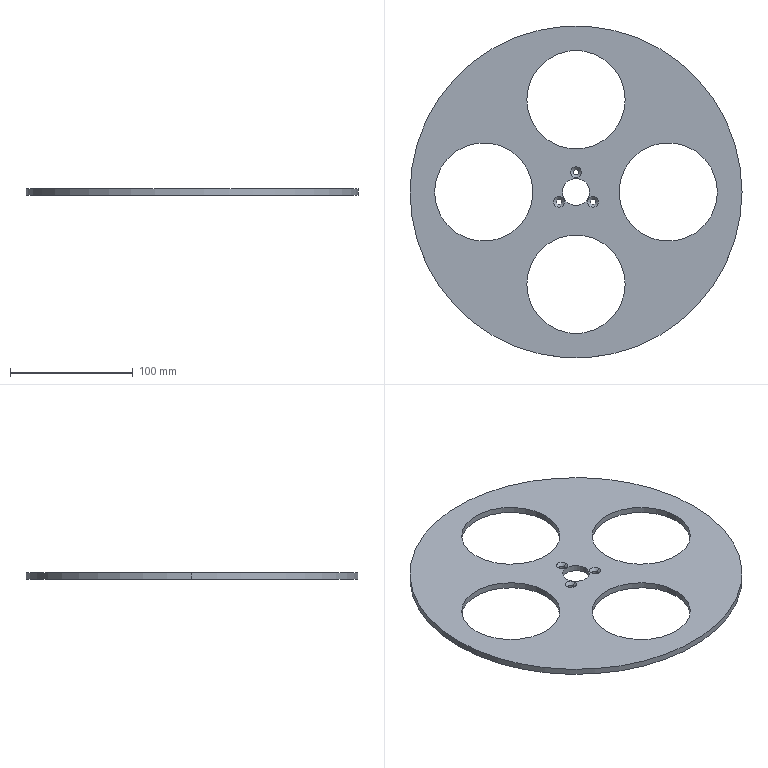Part | STEP file | QA-FC14 | 1 solid | 26 faces | box 270 x 270 x 5 mm | volume 183467 mm3 | cylinder 18 | cone 6 | plane 2 | commonest cylinder face diameters 80 x8 4.5 x6 22 x2 270 x2